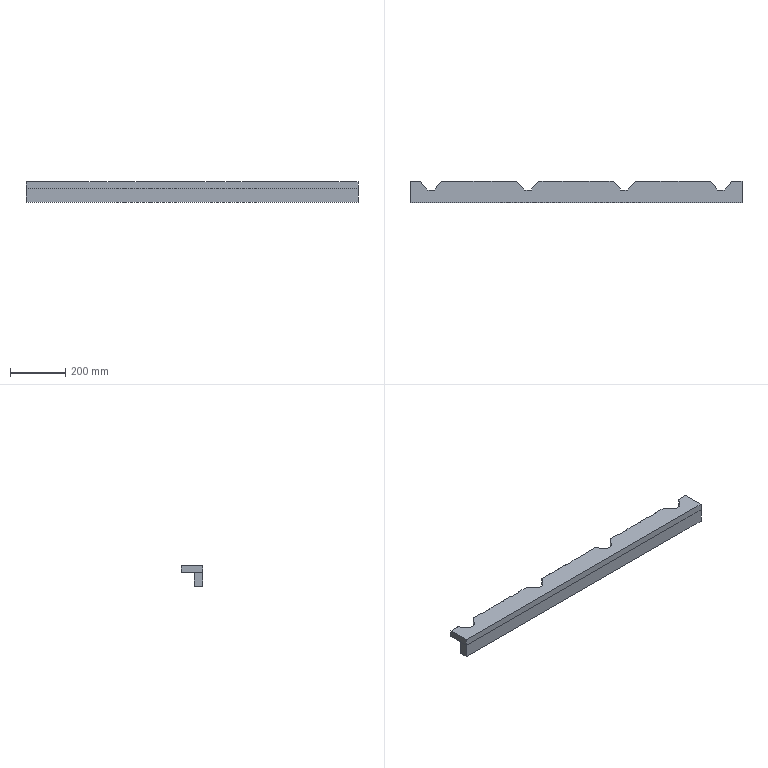Part | SolidWorks | features BaseBody 2 | 2 solids | 116 faces | box 1200 x 78 x 75 mm | volume 3953698 mm3 | plane 64 | cylinder 52 | commonest cylinder face diameters 6 x26 7 x26